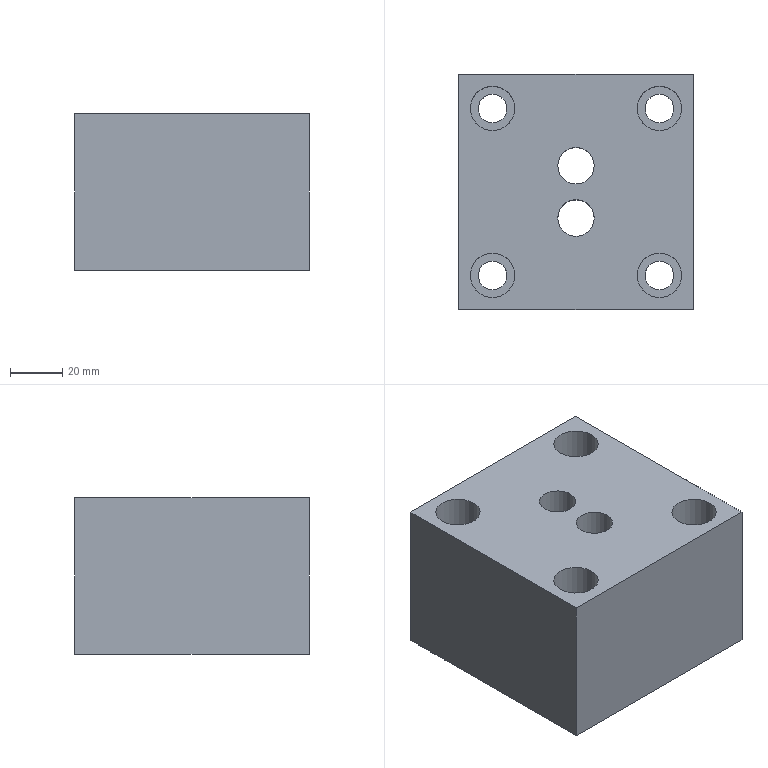Part | STEP file | PN_0007_id1774_x_t | 1 solid | 20 faces | box 90 x 90 x 60 mm | volume 428886 mm3 | plane 10 | cylinder 10 | commonest cylinder face diameters 11 x4 17 x4 14 x2
STEP:
#1=CARTESIAN_POINT('',(117.5,105.,155.));
#2=VERTEX_POINT('',#1);
#3=CARTESIAN_POINT('',(123.,105.,155.));
#4=DIRECTION('',(0.,0.,-1.));
#5=DIRECTION('',(-1.,0.,0.));
#6=AXIS2_PLACEMENT_3D('',#3,#4,#5);
#7=CIRCLE('',#6,5.5);
#8=EDGE_CURVE('',#2,#2,#7,.T.);
#9=ORIENTED_EDGE('',*,*,#8,.F.);
#10=EDGE_LOOP('',(#9));
#11=FACE_BOUND('',#10,.T.);
#12=CARTESIAN_POINT('',(117.5,169.,155.));
#13=VERTEX_POINT('',#12);
#14=CARTESIAN_POINT('',(123.,169.,155.));
#15=DIRECTION('',(0.,0.,1.));
#16=DIRECTION('',(-1.,0.,0.));
#17=AXIS2_PLACEMENT_3D('',#14,#15,#16);
#18=CIRCLE('',#17,5.5);
#19=EDGE_CURVE('',#13,#13,#18,.T.);
#20=ORIENTED_EDGE('',*,*,#19,.T.);
#21=EDGE_LOOP('',(#20));
#22=FACE_BOUND('',#21,.T.);
#23=CARTESIAN_POINT('',(64.5,105.,155.));
#24=VERTEX_POINT('',#23);
#25=CARTESIAN_POINT('',(59.,105.,155.));
#26=DIRECTION('',(0.,0.,1.));
#27=DIRECTION('',(1.,0.,0.));
#28=AXIS2_PLACEMENT_3D('',#25,#26,#27);
#29=CIRCLE('',#28,5.5);
#30=EDGE_CURVE('',#24,#24,#29,.T.);
#31=ORIENTED_EDGE('',*,*,#30,.T.);
#32=EDGE_LOOP('',(#31));
#33=FACE_BOUND('',#32,.T.);
#34=CARTESIAN_POINT('',(64.5,169.,155.));
#35=VERTEX_POINT('',#34);
#36=CARTESIAN_POINT('',(59.,169.,155.));
#37=DIRECTION('',(0.,0.,-1.));
#38=DIRECTION('',(1.,0.,0.));
#39=AXIS2_PLACEMENT_3D('',#36,#37,#38);
#40=CIRCLE('',#39,5.5);
#41=EDGE_CURVE('',#35,#35,#40,.T.);
#42=ORIENTED_EDGE('',*,*,#41,.F.);
#43=EDGE_LOOP('',(#42));
#44=FACE_BOUND('',#43,.T.);
#45=CARTESIAN_POINT('',(98.,127.,155.));
#46=VERTEX_POINT('',#45);
#47=CARTESIAN_POINT('',(91.,127.,155.));
#48=DIRECTION('',(0.,0.,1.));
#49=DIRECTION('',(1.,0.,0.));
#50=AXIS2_PLACEMENT_3D('',#47,#48,#49);
#51=CIRCLE('',#50,7.);
#52=EDGE_CURVE('',#46,#46,#51,.T.);
#53=ORIENTED_EDGE('',*,*,#52,.T.);
#54=EDGE_LOOP('',(#53));
#55=FACE_BOUND('',#54,.T.);
#56=CARTESIAN_POINT('',(98.,147.,155.));
#57=VERTEX_POINT('',#56);
#58=CARTESIAN_POINT('',(91.,147.,155.));
#59=DIRECTION('',(0.,0.,1.));
#60=DIRECTION('',(1.,0.,0.));
#61=AXIS2_PLACEMENT_3D('',#58,#59,#60);
#62=CIRCLE('',#61,7.);
#63=EDGE_CURVE('',#57,#57,#62,.T.);
#64=ORIENTED_EDGE('',*,*,#63,.T.);
#65=EDGE_LOOP('',(#64));
#66=FACE_BOUND('',#65,.T.);
#67=CARTESIAN_POINT('',(46.,92.,155.));
#68=VERTEX_POINT('',#67);
#69=CARTESIAN_POINT('',(136.,92.,155.));
#70=VERTEX_POINT('',#69);
#71=CARTESIAN_POINT('',(91.,92.,155.));
#72=DIRECTION('',(1.,0.,0.));
#73=VECTOR('',#72,1.);
#74=LINE('',#71,#73);
#75=EDGE_CURVE('',#68,#70,#74,.T.);
#76=ORIENTED_EDGE('',*,*,#75,.F.);
#77=CARTESIAN_POINT('',(46.,182.,155.));
#78=VERTEX_POINT('',#77);
#79=CARTESIAN_POINT('',(46.,69.6,155.));
#80=DIRECTION('',(0.,-1.,0.));
#81=VECTOR('',#80,1.);
#82=LINE('',#79,#81);
#83=EDGE_CURVE('',#78,#68,#82,.T.);
#84=ORIENTED_EDGE('',*,*,#83,.F.);
#85=CARTESIAN_POINT('',(136.,182.,155.));
#86=VERTEX_POINT('',#85);
#87=CARTESIAN_POINT('',(91.,182.,155.));
#88=DIRECTION('',(-1.,0.,0.));
#89=VECTOR('',#88,1.);
#90=LINE('',#87,#89);
#91=EDGE_CURVE('',#86,#78,#90,.T.);
#92=ORIENTED_EDGE('',*,*,#91,.F.);
#93=CARTESIAN_POINT('',(136.,137.,155.));
#94=DIRECTION('',(0.,1.,0.));
#95=VECTOR('',#94,1.);
#96=LINE('',#93,#95);
#97=EDGE_CURVE('',#70,#86,#96,.T.);
#98=ORIENTED_EDGE('',*,*,#97,.F.);
#99=EDGE_LOOP('',(#76,#84,#92,#98));
#100=FACE_BOUND('',#99,.T.);
#101=CARTESIAN_POINT('',(504.5,76.,155.));
#102=DIRECTION('',(0.,0.,-1.));
#103=DIRECTION('',(1.,0.,0.));
#104=AXIS2_PLACEMENT_3D('',#101,#102,#103);
#105=PLANE('',#104);
#106=ADVANCED_FACE('',(#11,#22,#33,#44,#55,#66,#100),#105,.T.);
#107=CARTESIAN_POINT('',(46.,92.,215.));
#108=VERTEX_POINT('',#107);
#109=CARTESIAN_POINT('',(46.,92.,155.));
#110=DIRECTION('',(0.,0.,-1.));
#111=VECTOR('',#110,1.);
#112=LINE('',#109,#111);
#113=EDGE_CURVE('',#108,#68,#112,.T.);
#114=ORIENTED_EDGE('',*,*,#113,.T.);
#115=ORIENTED_EDGE('',*,*,#75,.T.);
#116=CARTESIAN_POINT('',(136.,92.,215.));
#117=VERTEX_POINT('',#116);
#118=CARTESIAN_POINT('',(136.,92.,155.));
#119=DIRECTION('',(0.,0.,-1.));
#120=VECTOR('',#119,1.);
#121=LINE('',#118,#120);
#122=EDGE_CURVE('',#117,#70,#121,.T.);
#123=ORIENTED_EDGE('',*,*,#122,.F.);
#124=CARTESIAN_POINT('',(91.,92.,215.));
#125=DIRECTION('',(-1.,0.,0.));
#126=VECTOR('',#125,1.);
#127=LINE('',#124,#126);
#128=EDGE_CURVE('',#117,#108,#127,.T.);
#129=ORIENTED_EDGE('',*,*,#128,.T.);
#130=EDGE_LOOP('',(#114,#115,#123,#129));
#131=FACE_OUTER_BOUND('',#130,.T.);
#132=CARTESIAN_POINT('',(91.,92.,155.));
#133=DIRECTION('',(0.,-1.,0.));
#134=DIRECTION('',(0.,0.,-1.));
#135=AXIS2_PLACEMENT_3D('',#132,#133,#134);
#136=PLANE('',#135);
#137=ADVANCED_FACE('',(#131),#136,.T.);
#138=ORIENTED_EDGE('',*,*,#122,.T.);
#139=ORIENTED_EDGE('',*,*,#97,.T.);
#140=CARTESIAN_POINT('',(136.,182.,215.));
#141=VERTEX_POINT('',#140);
#142=CARTESIAN_POINT('',(136.,182.,155.));
#143=DIRECTION('',(0.,0.,-1.));
#144=VECTOR('',#143,1.);
#145=LINE('',#142,#144);
#146=EDGE_CURVE('',#141,#86,#145,.T.);
#147=ORIENTED_EDGE('',*,*,#146,.F.);
#148=CARTESIAN_POINT('',(136.,137.,215.));
#149=DIRECTION('',(0.,-1.,0.));
#150=VECTOR('',#149,1.);
#151=LINE('',#148,#150);
#152=EDGE_CURVE('',#141,#117,#151,.T.);
#153=ORIENTED_EDGE('',*,*,#152,.T.);
#154=EDGE_LOOP('',(#138,#139,#147,#153));
#155=FACE_OUTER_BOUND('',#154,.T.);
#156=CARTESIAN_POINT('',(136.,137.,155.));
#157=DIRECTION('',(1.,0.,0.));
#158=DIRECTION('',(0.,0.,-1.));
#159=AXIS2_PLACEMENT_3D('',#156,#157,#158);
#160=PLANE('',#159);
#161=ADVANCED_FACE('',(#155),#160,.T.);
#162=ORIENTED_EDGE('',*,*,#146,.T.);
#163=ORIENTED_EDGE('',*,*,#91,.T.);
#164=CARTESIAN_POINT('',(46.,182.,215.));
#165=VERTEX_POINT('',#164);
#166=CARTESIAN_POINT('',(46.,182.,138.004));
#167=DIRECTION('',(0.,0.,-1.));
#168=VECTOR('',#167,1.);
#169=LINE('',#166,#168);
#170=EDGE_CURVE('',#165,#78,#169,.T.);
#171=ORIENTED_EDGE('',*,*,#170,.F.);
#172=CARTESIAN_POINT('',(91.,182.,215.));
#173=DIRECTION('',(1.,0.,0.));
#174=VECTOR('',#173,1.);
#175=LINE('',#172,#174);
#176=EDGE_CURVE('',#165,#141,#175,.T.);
#177=ORIENTED_EDGE('',*,*,#176,.T.);
#178=EDGE_LOOP('',(#162,#163,#171,#177));
#179=FACE_OUTER_BOUND('',#178,.T.);
#180=CARTESIAN_POINT('',(91.,182.,155.));
#181=DIRECTION('',(0.,1.,0.));
#182=DIRECTION('',(0.,0.,1.));
#183=AXIS2_PLACEMENT_3D('',#180,#181,#182);
#184=PLANE('',#183);
#185=ADVANCED_FACE('',(#179),#184,.T.);
#186=CARTESIAN_POINT('',(131.5,105.,215.));
#187=VERTEX_POINT('',#186);
#188=CARTESIAN_POINT('',(123.,105.,215.));
#189=DIRECTION('',(0.,0.,1.));
#190=DIRECTION('',(1.,0.,0.));
#191=AXIS2_PLACEMENT_3D('',#188,#189,#190);
#192=CIRCLE('',#191,8.5);
#193=EDGE_CURVE('',#187,#187,#192,.T.);
#194=ORIENTED_EDGE('',*,*,#193,.F.);
#195=EDGE_LOOP('',(#194));
#196=FACE_BOUND('',#195,.T.);
#197=CARTESIAN_POINT('',(131.5,169.,215.));
#198=VERTEX_POINT('',#197);
#199=CARTESIAN_POINT('',(123.,169.,215.));
#200=DIRECTION('',(0.,0.,-1.));
#201=DIRECTION('',(1.,0.,0.));
#202=AXIS2_PLACEMENT_3D('',#199,#200,#201);
#203=CIRCLE('',#202,8.5);
#204=EDGE_CURVE('',#198,#198,#203,.T.);
#205=ORIENTED_EDGE('',*,*,#204,.T.);
#206=EDGE_LOOP('',(#205));
#207=FACE_BOUND('',#206,.T.);
#208=CARTESIAN_POINT('',(50.5,105.,215.));
#209=VERTEX_POINT('',#208);
#210=CARTESIAN_POINT('',(59.,105.,215.));
#211=DIRECTION('',(0.,0.,-1.));
#212=DIRECTION('',(-1.,0.,0.));
#213=AXIS2_PLACEMENT_3D('',#210,#211,#212);
#214=CIRCLE('',#213,8.5);
#215=EDGE_CURVE('',#209,#209,#214,.T.);
#216=ORIENTED_EDGE('',*,*,#215,.T.);
#217=EDGE_LOOP('',(#216));
#218=FACE_BOUND('',#217,.T.);
#219=CARTESIAN_POINT('',(50.5,169.,215.));
#220=VERTEX_POINT('',#219);
#221=CARTESIAN_POINT('',(59.,169.,215.));
#222=DIRECTION('',(0.,0.,1.));
#223=DIRECTION('',(-1.,0.,0.));
#224=AXIS2_PLACEMENT_3D('',#221,#222,#223);
#225=CIRCLE('',#224,8.5);
#226=EDGE_CURVE('',#220,#220,#225,.T.);
#227=ORIENTED_EDGE('',*,*,#226,.F.);
#228=EDGE_LOOP('',(#227));
#229=FACE_BOUND('',#228,.T.);
#230=CARTESIAN_POINT('',(84.,127.,215.));
#231=VERTEX_POINT('',#230);
#232=CARTESIAN_POINT('',(91.,127.,215.));
#233=DIRECTION('',(0.,0.,-1.));
#234=DIRECTION('',(-1.,0.,0.));
#235=AXIS2_PLACEMENT_3D('',#232,#233,#234);
#236=CIRCLE('',#235,7.);
#237=EDGE_CURVE('',#231,#231,#236,.T.);
#238=ORIENTED_EDGE('',*,*,#237,.T.);
#239=EDGE_LOOP('',(#238));
#240=FACE_BOUND('',#239,.T.);
#241=CARTESIAN_POINT('',(84.,147.,215.));
#242=VERTEX_POINT('',#241);
#243=CARTESIAN_POINT('',(91.,147.,215.));
#244=DIRECTION('',(0.,0.,-1.));
#245=DIRECTION('',(-1.,0.,0.));
#246=AXIS2_PLACEMENT_3D('',#243,#244,#245);
#247=CIRCLE('',#246,7.);
#248=EDGE_CURVE('',#242,#242,#247,.T.);
#249=ORIENTED_EDGE('',*,*,#248,.T.);
#250=EDGE_LOOP('',(#249));
#251=FACE_BOUND('',#250,.T.);
#252=CARTESIAN_POINT('',(46.,69.6,215.));
#253=DIRECTION('',(0.,1.,0.));
#254=VECTOR('',#253,1.);
#255=LINE('',#252,#254);
#256=EDGE_CURVE('',#108,#165,#255,.T.);
#257=ORIENTED_EDGE('',*,*,#256,.F.);
#258=ORIENTED_EDGE('',*,*,#128,.F.);
#259=ORIENTED_EDGE('',*,*,#152,.F.);
#260=ORIENTED_EDGE('',*,*,#176,.F.);
#261=EDGE_LOOP('',(#257,#258,#259,#260));
#262=FACE_BOUND('',#261,.T.);
#263=CARTESIAN_POINT('',(549.5,76.,215.));
#264=DIRECTION('',(0.,0.,-1.));
#265=DIRECTION('',(1.,0.,0.));
#266=AXIS2_PLACEMENT_3D('',#263,#264,#265);
#267=PLANE('',#266);
#268=ADVANCED_FACE('',(#196,#207,#218,#229,#240,#251,#262),#267,.F.);
#269=ORIENTED_EDGE('',*,*,#256,.T.);
#270=ORIENTED_EDGE('',*,*,#170,.T.);
#271=ORIENTED_EDGE('',*,*,#83,.T.);
#272=ORIENTED_EDGE('',*,*,#113,.F.);
#273=EDGE_LOOP('',(#269,#270,#271,#272));
#274=FACE_OUTER_BOUND('',#273,.T.);
#275=CARTESIAN_POINT('',(46.,69.6,138.004));
#276=DIRECTION('',(-1.,0.,0.));
#277=DIRECTION('',(0.,0.,-1.));
#278=AXIS2_PLACEMENT_3D('',#275,#276,#277);
#279=PLANE('',#278);
#280=ADVANCED_FACE('',(#274),#279,.T.);
#281=ORIENTED_EDGE('',*,*,#248,.F.);
#282=EDGE_LOOP('',(#281));
#283=FACE_BOUND('',#282,.T.);
#284=ORIENTED_EDGE('',*,*,#63,.F.);
#285=EDGE_LOOP('',(#284));
#286=FACE_BOUND('',#285,.T.);
#287=CARTESIAN_POINT('',(91.,147.,155.));
#288=DIRECTION('',(0.,0.,1.));
#289=DIRECTION('',(1.,0.,0.));
#290=AXIS2_PLACEMENT_3D('',#287,#288,#289);
#291=CYLINDRICAL_SURFACE('',#290,7.);
#292=ADVANCED_FACE('',(#283,#286),#291,.F.);
#293=ORIENTED_EDGE('',*,*,#237,.F.);
#294=EDGE_LOOP('',(#293));
#295=FACE_BOUND('',#294,.T.);
#296=ORIENTED_EDGE('',*,*,#52,.F.);
#297=EDGE_LOOP('',(#296));
#298=FACE_BOUND('',#297,.T.);
#299=CARTESIAN_POINT('',(91.,127.,155.));
#300=DIRECTION('',(0.,0.,1.));
#301=DIRECTION('',(1.,0.,0.));
#302=AXIS2_PLACEMENT_3D('',#299,#300,#301);
#303=CYLINDRICAL_SURFACE('',#302,7.);
#304=ADVANCED_FACE('',(#295,#298),#303,.F.);
#305=CARTESIAN_POINT('',(53.5,169.,185.));
#306=VERTEX_POINT('',#305);
#307=CARTESIAN_POINT('',(59.,169.,185.));
#308=DIRECTION('',(0.,0.,1.));
#309=DIRECTION('',(-1.,0.,0.));
#310=AXIS2_PLACEMENT_3D('',#307,#308,#309);
#311=CIRCLE('',#310,5.5);
#312=EDGE_CURVE('',#306,#306,#311,.T.);
#313=ORIENTED_EDGE('',*,*,#312,.T.);
#314=EDGE_LOOP('',(#313));
#315=FACE_BOUND('',#314,.T.);
#316=ORIENTED_EDGE('',*,*,#41,.T.);
#317=EDGE_LOOP('',(#316));
#318=FACE_BOUND('',#317,.T.);
#319=CARTESIAN_POINT('',(59.,169.,155.));
#320=DIRECTION('',(0.,0.,1.));
#321=DIRECTION('',(1.,0.,0.));
#322=AXIS2_PLACEMENT_3D('',#319,#320,#321);
#323=CYLINDRICAL_SURFACE('',#322,5.5);
#324=ADVANCED_FACE('',(#315,#318),#323,.F.);
#325=ORIENTED_EDGE('',*,*,#312,.F.);
#326=EDGE_LOOP('',(#325));
#327=FACE_BOUND('',#326,.T.);
#328=CARTESIAN_POINT('',(67.5,169.,185.));
#329=VERTEX_POINT('',#328);
#330=CARTESIAN_POINT('',(59.,169.,185.));
#331=DIRECTION('',(0.,0.,1.));
#332=DIRECTION('',(1.,0.,0.));
#333=AXIS2_PLACEMENT_3D('',#330,#331,#332);
#334=CIRCLE('',#333,8.5);
#335=EDGE_CURVE('',#329,#329,#334,.T.);
#336=ORIENTED_EDGE('',*,*,#335,.T.);
#337=EDGE_LOOP('',(#336));
#338=FACE_BOUND('',#337,.T.);
#339=CARTESIAN_POINT('',(59.,169.,185.));
#340=DIRECTION('',(0.,0.,-1.));
#341=DIRECTION('',(-1.,0.,0.));
#342=AXIS2_PLACEMENT_3D('',#339,#340,#341);
#343=PLANE('',#342);
#344=ADVANCED_FACE('',(#327,#338),#343,.F.);
#345=ORIENTED_EDGE('',*,*,#226,.T.);
#346=EDGE_LOOP('',(#345));
#347=FACE_BOUND('',#346,.T.);
#348=ORIENTED_EDGE('',*,*,#335,.F.);
#349=EDGE_LOOP('',(#348));
#350=FACE_BOUND('',#349,.T.);
#351=CARTESIAN_POINT('',(59.,169.,185.));
#352=DIRECTION('',(0.,0.,1.));
#353=DIRECTION('',(1.,0.,0.));
#354=AXIS2_PLACEMENT_3D('',#351,#352,#353);
#355=CYLINDRICAL_SURFACE('',#354,8.5);
#356=ADVANCED_FACE('',(#347,#350),#355,.F.);
#357=CARTESIAN_POINT('',(53.5,105.,185.));
#358=VERTEX_POINT('',#357);
#359=CARTESIAN_POINT('',(59.,105.,185.));
#360=DIRECTION('',(0.,0.,-1.));
#361=DIRECTION('',(-1.,0.,0.));
#362=AXIS2_PLACEMENT_3D('',#359,#360,#361);
#363=CIRCLE('',#362,5.5);
#364=EDGE_CURVE('',#358,#358,#363,.T.);
#365=ORIENTED_EDGE('',*,*,#364,.F.);
#366=EDGE_LOOP('',(#365));
#367=FACE_BOUND('',#366,.T.);
#368=ORIENTED_EDGE('',*,*,#30,.F.);
#369=EDGE_LOOP('',(#368));
#370=FACE_BOUND('',#369,.T.);
#371=CARTESIAN_POINT('',(59.,105.,155.));
#372=DIRECTION('',(0.,0.,1.));
#373=DIRECTION('',(1.,0.,0.));
#374=AXIS2_PLACEMENT_3D('',#371,#372,#373);
#375=CYLINDRICAL_SURFACE('',#374,5.5);
#376=ADVANCED_FACE('',(#367,#370),#375,.F.);
#377=ORIENTED_EDGE('',*,*,#364,.T.);
#378=EDGE_LOOP('',(#377));
#379=FACE_BOUND('',#378,.T.);
#380=CARTESIAN_POINT('',(67.5,105.,185.));
#381=VERTEX_POINT('',#380);
#382=CARTESIAN_POINT('',(59.,105.,185.));
#383=DIRECTION('',(0.,0.,-1.));
#384=DIRECTION('',(1.,0.,0.));
#385=AXIS2_PLACEMENT_3D('',#382,#383,#384);
#386=CIRCLE('',#385,8.5);
#387=EDGE_CURVE('',#381,#381,#386,.T.);
#388=ORIENTED_EDGE('',*,*,#387,.F.);
#389=EDGE_LOOP('',(#388));
#390=FACE_BOUND('',#389,.T.);
#391=CARTESIAN_POINT('',(59.,105.,185.));
#392=DIRECTION('',(0.,0.,-1.));
#393=DIRECTION('',(-1.,0.,0.));
#394=AXIS2_PLACEMENT_3D('',#391,#392,#393);
#395=PLANE('',#394);
#396=ADVANCED_FACE('',(#379,#390),#395,.F.);
#397=ORIENTED_EDGE('',*,*,#215,.F.);
#398=EDGE_LOOP('',(#397));
#399=FACE_BOUND('',#398,.T.);
#400=ORIENTED_EDGE('',*,*,#387,.T.);
#401=EDGE_LOOP('',(#400));
#402=FACE_BOUND('',#401,.T.);
#403=CARTESIAN_POINT('',(59.,105.,185.));
#404=DIRECTION('',(0.,0.,1.));
#405=DIRECTION('',(1.,0.,0.));
#406=AXIS2_PLACEMENT_3D('',#403,#404,#405);
#407=CYLINDRICAL_SURFACE('',#406,8.5);
#408=ADVANCED_FACE('',(#399,#402),#407,.F.);
#409=CARTESIAN_POINT('',(128.5,169.,185.));
#410=VERTEX_POINT('',#409);
#411=CARTESIAN_POINT('',(123.,169.,185.));
#412=DIRECTION('',(0.,0.,-1.));
#413=DIRECTION('',(1.,0.,0.));
#414=AXIS2_PLACEMENT_3D('',#411,#412,#413);
#415=CIRCLE('',#414,5.5);
#416=EDGE_CURVE('',#410,#410,#415,.T.);
#417=ORIENTED_EDGE('',*,*,#416,.F.);
#418=EDGE_LOOP('',(#417));
#419=FACE_BOUND('',#418,.T.);
#420=ORIENTED_EDGE('',*,*,#19,.F.);
#421=EDGE_LOOP('',(#420));
#422=FACE_BOUND('',#421,.T.);
#423=CARTESIAN_POINT('',(123.,169.,155.));
#424=DIRECTION('',(0.,0.,1.));
#425=DIRECTION('',(-1.,0.,0.));
#426=AXIS2_PLACEMENT_3D('',#423,#424,#425);
#427=CYLINDRICAL_SURFACE('',#426,5.5);
#428=ADVANCED_FACE('',(#419,#422),#427,.F.);
#429=ORIENTED_EDGE('',*,*,#416,.T.);
#430=EDGE_LOOP('',(#429));
#431=FACE_BOUND('',#430,.T.);
#432=CARTESIAN_POINT('',(114.5,169.,185.));
#433=VERTEX_POINT('',#432);
#434=CARTESIAN_POINT('',(123.,169.,185.));
#435=DIRECTION('',(0.,0.,-1.));
#436=DIRECTION('',(-1.,0.,0.));
#437=AXIS2_PLACEMENT_3D('',#434,#435,#436);
#438=CIRCLE('',#437,8.5);
#439=EDGE_CURVE('',#433,#433,#438,.T.);
#440=ORIENTED_EDGE('',*,*,#439,.F.);
#441=EDGE_LOOP('',(#440));
#442=FACE_BOUND('',#441,.T.);
#443=CARTESIAN_POINT('',(123.,169.,185.));
#444=DIRECTION('',(0.,0.,-1.));
#445=DIRECTION('',(1.,0.,0.));
#446=AXIS2_PLACEMENT_3D('',#443,#444,#445);
#447=PLANE('',#446);
#448=ADVANCED_FACE('',(#431,#442),#447,.F.);
#449=ORIENTED_EDGE('',*,*,#204,.F.);
#450=EDGE_LOOP('',(#449));
#451=FACE_BOUND('',#450,.T.);
#452=ORIENTED_EDGE('',*,*,#439,.T.);
#453=EDGE_LOOP('',(#452));
#454=FACE_BOUND('',#453,.T.);
#455=CARTESIAN_POINT('',(123.,169.,185.));
#456=DIRECTION('',(0.,0.,1.));
#457=DIRECTION('',(-1.,0.,0.));
#458=AXIS2_PLACEMENT_3D('',#455,#456,#457);
#459=CYLINDRICAL_SURFACE('',#458,8.5);
#460=ADVANCED_FACE('',(#451,#454),#459,.F.);
#461=CARTESIAN_POINT('',(128.5,105.,185.));
#462=VERTEX_POINT('',#461);
#463=CARTESIAN_POINT('',(123.,105.,185.));
#464=DIRECTION('',(0.,0.,1.));
#465=DIRECTION('',(1.,0.,0.));
#466=AXIS2_PLACEMENT_3D('',#463,#464,#465);
#467=CIRCLE('',#466,5.5);
#468=EDGE_CURVE('',#462,#462,#467,.T.);
#469=ORIENTED_EDGE('',*,*,#468,.T.);
#470=EDGE_LOOP('',(#469));
#471=FACE_BOUND('',#470,.T.);
#472=ORIENTED_EDGE('',*,*,#8,.T.);
#473=EDGE_LOOP('',(#472));
#474=FACE_BOUND('',#473,.T.);
#475=CARTESIAN_POINT('',(123.,105.,155.));
#476=DIRECTION('',(0.,0.,1.));
#477=DIRECTION('',(-1.,0.,0.));
#478=AXIS2_PLACEMENT_3D('',#475,#476,#477);
#479=CYLINDRICAL_SURFACE('',#478,5.5);
#480=ADVANCED_FACE('',(#471,#474),#479,.F.);
#481=ORIENTED_EDGE('',*,*,#468,.F.);
#482=EDGE_LOOP('',(#481));
#483=FACE_BOUND('',#482,.T.);
#484=CARTESIAN_POINT('',(114.5,105.,185.));
#485=VERTEX_POINT('',#484);
#486=CARTESIAN_POINT('',(123.,105.,185.));
#487=DIRECTION('',(0.,0.,1.));
#488=DIRECTION('',(-1.,0.,0.));
#489=AXIS2_PLACEMENT_3D('',#486,#487,#488);
#490=CIRCLE('',#489,8.5);
#491=EDGE_CURVE('',#485,#485,#490,.T.);
#492=ORIENTED_EDGE('',*,*,#491,.T.);
#493=EDGE_LOOP('',(#492));
#494=FACE_BOUND('',#493,.T.);
#495=CARTESIAN_POINT('',(123.,105.,185.));
#496=DIRECTION('',(0.,0.,-1.));
#497=DIRECTION('',(1.,0.,0.));
#498=AXIS2_PLACEMENT_3D('',#495,#496,#497);
#499=PLANE('',#498);
#500=ADVANCED_FACE('',(#483,#494),#499,.F.);
#501=ORIENTED_EDGE('',*,*,#193,.T.);
#502=EDGE_LOOP('',(#501));
#503=FACE_BOUND('',#502,.T.);
#504=ORIENTED_EDGE('',*,*,#491,.F.);
#505=EDGE_LOOP('',(#504));
#506=FACE_BOUND('',#505,.T.);
#507=CARTESIAN_POINT('',(123.,105.,185.));
#508=DIRECTION('',(0.,0.,1.));
#509=DIRECTION('',(-1.,0.,0.));
#510=AXIS2_PLACEMENT_3D('',#507,#508,#509);
#511=CYLINDRICAL_SURFACE('',#510,8.5);
#512=ADVANCED_FACE('',(#503,#506),#511,.F.);
#513=CLOSED_SHELL('',(#106,#137,#161,#185,#268,#280,#292,#304,#324,#344,#356,#376,#396,#408,#428,#448,#460,#480,#500,#512));
#514=MANIFOLD_SOLID_BREP('',#513);
#515=(LENGTH_UNIT()NAMED_UNIT(*)SI_UNIT(.MILLI.,.METRE.));
#516=UNCERTAINTY_MEASURE_WITH_UNIT(LENGTH_MEASURE(0.00002),#515,'','');
#517=(NAMED_UNIT(*)PLANE_ANGLE_UNIT()SI_UNIT($,.RADIAN.));
#518=PLANE_ANGLE_MEASURE_WITH_UNIT(PLANE_ANGLE_MEASURE(0.01745),#517);
#519=DIMENSIONAL_EXPONENTS(0.,0.,0.,0.,0.,0.,0.);
#520=(CONVERSION_BASED_UNIT('DEGREE',#518)NAMED_UNIT(#519)PLANE_ANGLE_UNIT());
#521=(NAMED_UNIT(*)SI_UNIT($,.STERADIAN.)SOLID_ANGLE_UNIT());
#522=(GEOMETRIC_REPRESENTATION_CONTEXT(3)GLOBAL_UNCERTAINTY_ASSIGNED_CONTEXT((#516))GLOBAL_UNIT_ASSIGNED_CONTEXT((#515,#520,#521))REPRESENTATION_CONTEXT('',''));
#523=ADVANCED_BREP_SHAPE_REPRESENTATION('',(#514),#522);